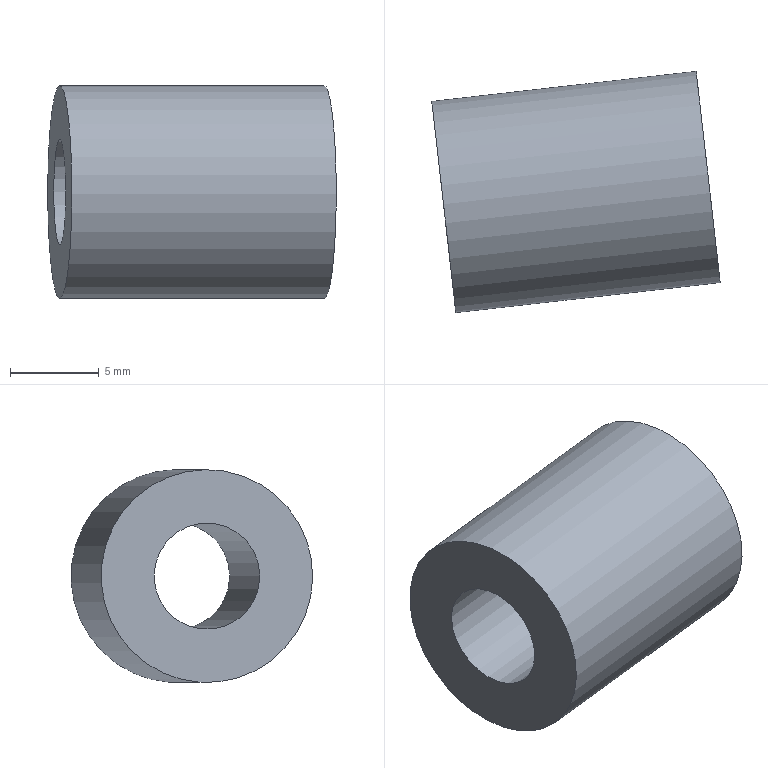Part | NX | features solid 2 | 1 solid | 4 faces | box 16.262 x 13.621 x 12 mm | volume 1272 mm3 | plane 2 | cylinder 2 | commonest cylinder face diameters 6.001 x1 12 x1
STEP:
#1=CARTESIAN_POINT('',(2683.045,190.657,-48.416));
#2=VERTEX_POINT('',#1);
#3=CARTESIAN_POINT('',(2682.706,193.639,-48.416));
#4=DIRECTION('',(0.9936,0.1132,0.000000001));
#5=DIRECTION('',(0.1132,-0.9936,0.));
#6=AXIS2_PLACEMENT_3D('',#3,#4,#5);
#7=CIRCLE('',#6,3.001);
#8=EDGE_CURVE('',#2,#2,#7,.T.);
#9=ORIENTED_EDGE('',*,*,#8,.F.);
#10=EDGE_LOOP('',(#9));
#11=FACE_BOUND('',#10,.T.);
#12=CARTESIAN_POINT('',(2682.783,192.964,-54.377));
#13=VERTEX_POINT('',#12);
#14=CARTESIAN_POINT('',(2682.706,193.639,-48.416));
#15=DIRECTION('',(0.9936,0.1132,0.000000001));
#16=DIRECTION('',(0.01281,-0.1125,-0.9936));
#17=AXIS2_PLACEMENT_3D('',#14,#15,#16);
#18=CIRCLE('',#17,6.);
#19=EDGE_CURVE('',#13,#13,#18,.T.);
#20=ORIENTED_EDGE('',*,*,#19,.T.);
#21=EDGE_LOOP('',(#20));
#22=FACE_BOUND('',#21,.T.);
#23=CARTESIAN_POINT('',(2682.706,193.639,-48.416));
#24=DIRECTION('',(0.9936,0.1132,0.000000001));
#25=DIRECTION('',(-0.1132,0.9936,0.));
#26=AXIS2_PLACEMENT_3D('',#23,#24,#25);
#27=PLANE('',#26);
#28=ADVANCED_FACE('',(#11,#22),#27,.T.);
#29=CARTESIAN_POINT('',(2667.463,194.922,-48.416));
#30=VERTEX_POINT('',#29);
#31=CARTESIAN_POINT('',(2667.802,191.94,-48.416));
#32=DIRECTION('',(-0.9936,-0.1132,-0.000000001));
#33=DIRECTION('',(-0.1132,0.9936,0.));
#34=AXIS2_PLACEMENT_3D('',#31,#32,#33);
#35=CIRCLE('',#34,3.001);
#36=EDGE_CURVE('',#30,#30,#35,.T.);
#37=ORIENTED_EDGE('',*,*,#36,.F.);
#38=EDGE_LOOP('',(#37));
#39=FACE_BOUND('',#38,.T.);
#40=CARTESIAN_POINT('',(2667.879,191.266,-54.377));
#41=VERTEX_POINT('',#40);
#42=CARTESIAN_POINT('',(2667.802,191.94,-48.416));
#43=DIRECTION('',(-0.9936,-0.1132,-0.000000001));
#44=DIRECTION('',(0.01281,-0.1125,-0.9936));
#45=AXIS2_PLACEMENT_3D('',#42,#43,#44);
#46=CIRCLE('',#45,6.);
#47=EDGE_CURVE('',#41,#41,#46,.T.);
#48=ORIENTED_EDGE('',*,*,#47,.T.);
#49=EDGE_LOOP('',(#48));
#50=FACE_BOUND('',#49,.T.);
#51=CARTESIAN_POINT('',(2667.802,191.94,-48.416));
#52=DIRECTION('',(-0.9936,-0.1132,-0.000000001));
#53=DIRECTION('',(0.1132,-0.9936,0.));
#54=AXIS2_PLACEMENT_3D('',#51,#52,#53);
#55=PLANE('',#54);
#56=ADVANCED_FACE('',(#39,#50),#55,.T.);
#57=ORIENTED_EDGE('',*,*,#19,.F.);
#58=EDGE_LOOP('',(#57));
#59=FACE_BOUND('',#58,.T.);
#60=ORIENTED_EDGE('',*,*,#47,.F.);
#61=EDGE_LOOP('',(#60));
#62=FACE_BOUND('',#61,.T.);
#63=CARTESIAN_POINT('',(2667.802,191.94,-48.416));
#64=DIRECTION('',(0.9936,0.1132,0.000000001));
#65=DIRECTION('',(-0.01281,0.1125,0.9936));
#66=AXIS2_PLACEMENT_3D('',#63,#64,#65);
#67=CYLINDRICAL_SURFACE('',#66,6.);
#68=ADVANCED_FACE('',(#59,#62),#67,.T.);
#69=ORIENTED_EDGE('',*,*,#8,.T.);
#70=EDGE_LOOP('',(#69));
#71=FACE_BOUND('',#70,.T.);
#72=ORIENTED_EDGE('',*,*,#36,.T.);
#73=EDGE_LOOP('',(#72));
#74=FACE_BOUND('',#73,.T.);
#75=CARTESIAN_POINT('',(7948.401,793.589,-48.416));
#76=DIRECTION('',(-0.9936,-0.1132,-0.000000001));
#77=DIRECTION('',(0.1132,-0.9936,0.));
#78=AXIS2_PLACEMENT_3D('',#75,#76,#77);
#79=CYLINDRICAL_SURFACE('',#78,3.001);
#80=ADVANCED_FACE('',(#71,#74),#79,.F.);
#81=CLOSED_SHELL('',(#28,#56,#68,#80));
#82=MANIFOLD_SOLID_BREP('',#81);
#83=(LENGTH_UNIT()NAMED_UNIT(*)SI_UNIT(.MILLI.,.METRE.));
#84=UNCERTAINTY_MEASURE_WITH_UNIT(LENGTH_MEASURE(0.00001),#83,'','');
#85=(NAMED_UNIT(*)PLANE_ANGLE_UNIT()SI_UNIT($,.RADIAN.));
#86=(NAMED_UNIT(*)SI_UNIT($,.STERADIAN.)SOLID_ANGLE_UNIT());
#87=(GEOMETRIC_REPRESENTATION_CONTEXT(3)GLOBAL_UNCERTAINTY_ASSIGNED_CONTEXT((#84))GLOBAL_UNIT_ASSIGNED_CONTEXT((#83,#85,#86))REPRESENTATION_CONTEXT('',''));
#88=ADVANCED_BREP_SHAPE_REPRESENTATION('',(#82),#87);